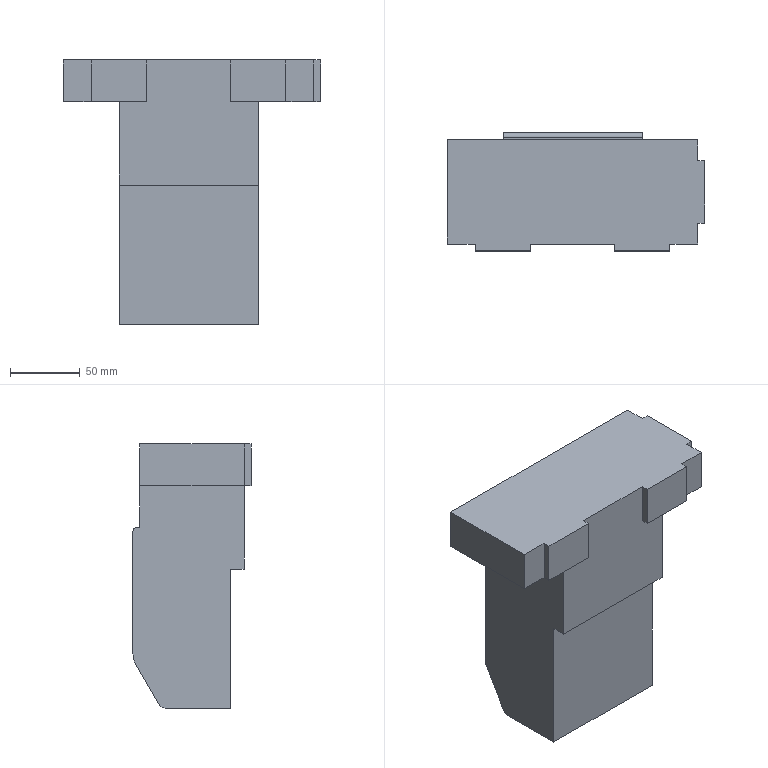Part | NX | features solid 2 | 1 solid | 30 faces | box 185 x 85 x 190 mm | volume 1552921 mm3 | plane 27 | cylinder 3 | commonest cylinder face diameters 6 x1 10 x1 30 x1
STEP:
#1=CARTESIAN_POINT('',(510.,415.,-90.));
#2=VERTEX_POINT('',#1);
#3=CARTESIAN_POINT('',(510.,415.,-120.));
#4=VERTEX_POINT('',#3);
#5=CARTESIAN_POINT('',(510.,415.,-90.));
#6=DIRECTION('',(0.,0.,-1.));
#7=VECTOR('',#6,1000.);
#8=LINE('',#5,#7);
#9=EDGE_CURVE('',#2,#4,#8,.T.);
#10=ORIENTED_EDGE('',*,*,#9,.F.);
#11=CARTESIAN_POINT('',(510.,400.,-90.));
#12=VERTEX_POINT('',#11);
#13=CARTESIAN_POINT('',(510.,475.,-90.));
#14=DIRECTION('',(0.,1.,0.));
#15=VECTOR('',#14,1000.);
#16=LINE('',#13,#15);
#17=EDGE_CURVE('',#2,#12,#16,.F.);
#18=ORIENTED_EDGE('',*,*,#17,.T.);
#19=CARTESIAN_POINT('',(510.,400.,-120.));
#20=VERTEX_POINT('',#19);
#21=CARTESIAN_POINT('',(510.,400.,-90.));
#22=DIRECTION('',(0.,0.,-1.));
#23=VECTOR('',#22,1000.);
#24=LINE('',#21,#23);
#25=EDGE_CURVE('',#12,#20,#24,.T.);
#26=ORIENTED_EDGE('',*,*,#25,.T.);
#27=CARTESIAN_POINT('',(510.,475.,-120.));
#28=DIRECTION('',(0.,1.,0.));
#29=VECTOR('',#28,1000.);
#30=LINE('',#27,#29);
#31=EDGE_CURVE('',#4,#20,#30,.F.);
#32=ORIENTED_EDGE('',*,*,#31,.F.);
#33=EDGE_LOOP('',(#10,#18,#26,#32));
#34=FACE_BOUND('',#33,.T.);
#35=CARTESIAN_POINT('',(510.,475.,-90.));
#36=DIRECTION('',(-1.,0.,0.));
#37=DIRECTION('',(0.,0.,-1.));
#38=AXIS2_PLACEMENT_3D('',#35,#36,#37);
#39=PLANE('',#38);
#40=ADVANCED_FACE('',(#34),#39,.F.);
#41=CARTESIAN_POINT('',(490.,400.,-120.));
#42=VERTEX_POINT('',#41);
#43=CARTESIAN_POINT('',(490.,400.,-90.));
#44=VERTEX_POINT('',#43);
#45=CARTESIAN_POINT('',(490.,400.,-180.));
#46=DIRECTION('',(0.,0.,1.));
#47=VECTOR('',#46,1000.);
#48=LINE('',#45,#47);
#49=EDGE_CURVE('',#42,#44,#48,.T.);
#50=ORIENTED_EDGE('',*,*,#49,.F.);
#51=CARTESIAN_POINT('',(470.,400.,-120.));
#52=DIRECTION('',(1.,0.,0.));
#53=VECTOR('',#52,1000.);
#54=LINE('',#51,#53);
#55=EDGE_CURVE('',#20,#42,#54,.F.);
#56=ORIENTED_EDGE('',*,*,#55,.F.);
#57=ORIENTED_EDGE('',*,*,#25,.F.);
#58=CARTESIAN_POINT('',(370.,400.,-90.));
#59=DIRECTION('',(1.,0.,0.));
#60=VECTOR('',#59,1000.);
#61=LINE('',#58,#60);
#62=EDGE_CURVE('',#44,#12,#61,.T.);
#63=ORIENTED_EDGE('',*,*,#62,.F.);
#64=EDGE_LOOP('',(#50,#56,#57,#63));
#65=FACE_BOUND('',#64,.T.);
#66=CARTESIAN_POINT('',(370.,400.,-180.));
#67=DIRECTION('',(0.,-1.,0.));
#68=DIRECTION('',(0.,0.,-1.));
#69=AXIS2_PLACEMENT_3D('',#66,#67,#68);
#70=PLANE('',#69);
#71=ADVANCED_FACE('',(#65),#70,.T.);
#72=CARTESIAN_POINT('',(330.,475.,-90.));
#73=VERTEX_POINT('',#72);
#74=CARTESIAN_POINT('',(510.,475.,-90.));
#75=VERTEX_POINT('',#74);
#76=CARTESIAN_POINT('',(370.,475.,-90.));
#77=DIRECTION('',(1.,0.,0.));
#78=VECTOR('',#77,1000.);
#79=LINE('',#76,#78);
#80=EDGE_CURVE('',#73,#75,#79,.T.);
#81=ORIENTED_EDGE('',*,*,#80,.T.);
#82=CARTESIAN_POINT('',(510.,475.,-120.));
#83=VERTEX_POINT('',#82);
#84=CARTESIAN_POINT('',(510.,475.,-90.));
#85=DIRECTION('',(0.,0.,-1.));
#86=VECTOR('',#85,1000.);
#87=LINE('',#84,#86);
#88=EDGE_CURVE('',#75,#83,#87,.T.);
#89=ORIENTED_EDGE('',*,*,#88,.T.);
#90=CARTESIAN_POINT('',(470.,475.,-120.));
#91=VERTEX_POINT('',#90);
#92=CARTESIAN_POINT('',(470.,475.,-120.));
#93=DIRECTION('',(1.,0.,0.));
#94=VECTOR('',#93,1000.);
#95=LINE('',#92,#94);
#96=EDGE_CURVE('',#83,#91,#95,.F.);
#97=ORIENTED_EDGE('',*,*,#96,.T.);
#98=CARTESIAN_POINT('',(470.,475.,-150.));
#99=VERTEX_POINT('',#98);
#100=CARTESIAN_POINT('',(470.,475.,-90.));
#101=DIRECTION('',(0.,0.,-1.));
#102=VECTOR('',#101,1000.);
#103=LINE('',#100,#102);
#104=EDGE_CURVE('',#91,#99,#103,.T.);
#105=ORIENTED_EDGE('',*,*,#104,.T.);
#106=CARTESIAN_POINT('',(370.,475.,-150.));
#107=VERTEX_POINT('',#106);
#108=CARTESIAN_POINT('',(370.,475.,-150.));
#109=DIRECTION('',(1.,0.,0.));
#110=VECTOR('',#109,1000.);
#111=LINE('',#108,#110);
#112=EDGE_CURVE('',#107,#99,#111,.T.);
#113=ORIENTED_EDGE('',*,*,#112,.F.);
#114=CARTESIAN_POINT('',(370.,475.,-120.));
#115=VERTEX_POINT('',#114);
#116=CARTESIAN_POINT('',(370.,475.,-90.));
#117=DIRECTION('',(0.,0.,-1.));
#118=VECTOR('',#117,1000.);
#119=LINE('',#116,#118);
#120=EDGE_CURVE('',#115,#107,#119,.T.);
#121=ORIENTED_EDGE('',*,*,#120,.F.);
#122=CARTESIAN_POINT('',(330.,475.,-120.));
#123=VERTEX_POINT('',#122);
#124=CARTESIAN_POINT('',(370.,475.,-120.));
#125=DIRECTION('',(1.,0.,0.));
#126=VECTOR('',#125,1000.);
#127=LINE('',#124,#126);
#128=EDGE_CURVE('',#123,#115,#127,.T.);
#129=ORIENTED_EDGE('',*,*,#128,.F.);
#130=CARTESIAN_POINT('',(330.,475.,-90.));
#131=DIRECTION('',(0.,0.,-1.));
#132=VECTOR('',#131,1000.);
#133=LINE('',#130,#132);
#134=EDGE_CURVE('',#73,#123,#133,.T.);
#135=ORIENTED_EDGE('',*,*,#134,.F.);
#136=EDGE_LOOP('',(#81,#89,#97,#105,#113,#121,#129,#135));
#137=FACE_BOUND('',#136,.T.);
#138=CARTESIAN_POINT('',(370.,475.,-90.));
#139=DIRECTION('',(0.,1.,0.));
#140=DIRECTION('',(0.,0.,1.));
#141=AXIS2_PLACEMENT_3D('',#138,#139,#140);
#142=PLANE('',#141);
#143=ADVANCED_FACE('',(#137),#142,.T.);
#144=ORIENTED_EDGE('',*,*,#80,.F.);
#145=CARTESIAN_POINT('',(330.,400.,-90.));
#146=VERTEX_POINT('',#145);
#147=CARTESIAN_POINT('',(330.,475.,-90.));
#148=DIRECTION('',(0.,1.,0.));
#149=VECTOR('',#148,1000.);
#150=LINE('',#147,#149);
#151=EDGE_CURVE('',#73,#146,#150,.F.);
#152=ORIENTED_EDGE('',*,*,#151,.T.);
#153=CARTESIAN_POINT('',(350.,400.,-90.));
#154=VERTEX_POINT('',#153);
#155=CARTESIAN_POINT('',(370.,400.,-90.));
#156=DIRECTION('',(1.,0.,0.));
#157=VECTOR('',#156,1000.);
#158=LINE('',#155,#157);
#159=EDGE_CURVE('',#146,#154,#158,.T.);
#160=ORIENTED_EDGE('',*,*,#159,.T.);
#161=CARTESIAN_POINT('',(350.,395.,-90.));
#162=VERTEX_POINT('',#161);
#163=CARTESIAN_POINT('',(350.,395.,-90.));
#164=DIRECTION('',(0.,1.,0.));
#165=VECTOR('',#164,1000.);
#166=LINE('',#163,#165);
#167=EDGE_CURVE('',#162,#154,#166,.T.);
#168=ORIENTED_EDGE('',*,*,#167,.F.);
#169=CARTESIAN_POINT('',(390.,395.,-90.));
#170=VERTEX_POINT('',#169);
#171=CARTESIAN_POINT('',(290.,395.,-90.));
#172=DIRECTION('',(1.,0.,0.));
#173=VECTOR('',#172,1000.);
#174=LINE('',#171,#173);
#175=EDGE_CURVE('',#162,#170,#174,.T.);
#176=ORIENTED_EDGE('',*,*,#175,.T.);
#177=CARTESIAN_POINT('',(390.,400.,-90.));
#178=VERTEX_POINT('',#177);
#179=CARTESIAN_POINT('',(390.,395.,-90.));
#180=DIRECTION('',(0.,1.,0.));
#181=VECTOR('',#180,1000.);
#182=LINE('',#179,#181);
#183=EDGE_CURVE('',#170,#178,#182,.T.);
#184=ORIENTED_EDGE('',*,*,#183,.T.);
#185=CARTESIAN_POINT('',(450.,400.,-90.));
#186=VERTEX_POINT('',#185);
#187=CARTESIAN_POINT('',(370.,400.,-90.));
#188=DIRECTION('',(1.,0.,0.));
#189=VECTOR('',#188,1000.);
#190=LINE('',#187,#189);
#191=EDGE_CURVE('',#178,#186,#190,.T.);
#192=ORIENTED_EDGE('',*,*,#191,.T.);
#193=CARTESIAN_POINT('',(450.,395.,-90.));
#194=VERTEX_POINT('',#193);
#195=CARTESIAN_POINT('',(450.,395.,-90.));
#196=DIRECTION('',(0.,1.,0.));
#197=VECTOR('',#196,1000.);
#198=LINE('',#195,#197);
#199=EDGE_CURVE('',#194,#186,#198,.T.);
#200=ORIENTED_EDGE('',*,*,#199,.F.);
#201=CARTESIAN_POINT('',(490.,395.,-90.));
#202=VERTEX_POINT('',#201);
#203=CARTESIAN_POINT('',(390.,395.,-90.));
#204=DIRECTION('',(1.,0.,0.));
#205=VECTOR('',#204,1000.);
#206=LINE('',#203,#205);
#207=EDGE_CURVE('',#194,#202,#206,.T.);
#208=ORIENTED_EDGE('',*,*,#207,.T.);
#209=CARTESIAN_POINT('',(490.,395.,-90.));
#210=DIRECTION('',(0.,1.,0.));
#211=VECTOR('',#210,1000.);
#212=LINE('',#209,#211);
#213=EDGE_CURVE('',#202,#44,#212,.T.);
#214=ORIENTED_EDGE('',*,*,#213,.T.);
#215=ORIENTED_EDGE('',*,*,#62,.T.);
#216=ORIENTED_EDGE('',*,*,#17,.F.);
#217=CARTESIAN_POINT('',(515.,415.,-90.));
#218=VERTEX_POINT('',#217);
#219=CARTESIAN_POINT('',(515.,415.,-90.));
#220=DIRECTION('',(-1.,0.,0.));
#221=VECTOR('',#220,1000.);
#222=LINE('',#219,#221);
#223=EDGE_CURVE('',#218,#2,#222,.T.);
#224=ORIENTED_EDGE('',*,*,#223,.F.);
#225=CARTESIAN_POINT('',(515.,460.,-90.));
#226=VERTEX_POINT('',#225);
#227=CARTESIAN_POINT('',(515.,475.,-90.));
#228=DIRECTION('',(0.,1.,0.));
#229=VECTOR('',#228,1000.);
#230=LINE('',#227,#229);
#231=EDGE_CURVE('',#226,#218,#230,.F.);
#232=ORIENTED_EDGE('',*,*,#231,.F.);
#233=CARTESIAN_POINT('',(510.,460.,-90.));
#234=VERTEX_POINT('',#233);
#235=CARTESIAN_POINT('',(515.,460.,-90.));
#236=DIRECTION('',(-1.,0.,0.));
#237=VECTOR('',#236,1000.);
#238=LINE('',#235,#237);
#239=EDGE_CURVE('',#226,#234,#238,.T.);
#240=ORIENTED_EDGE('',*,*,#239,.T.);
#241=CARTESIAN_POINT('',(510.,475.,-90.));
#242=DIRECTION('',(0.,1.,0.));
#243=VECTOR('',#242,1000.);
#244=LINE('',#241,#243);
#245=EDGE_CURVE('',#75,#234,#244,.F.);
#246=ORIENTED_EDGE('',*,*,#245,.F.);
#247=EDGE_LOOP('',(#144,#152,#160,#168,#176,#184,#192,#200,#208,#214,#215,#216,#224,#232,#240,#246));
#248=FACE_BOUND('',#247,.T.);
#249=CARTESIAN_POINT('',(370.,475.,-90.));
#250=DIRECTION('',(0.,0.,-1.));
#251=DIRECTION('',(1.,0.,0.));
#252=AXIS2_PLACEMENT_3D('',#249,#250,#251);
#253=PLANE('',#252);
#254=ADVANCED_FACE('',(#248),#253,.F.);
#255=CARTESIAN_POINT('',(390.,400.,-120.));
#256=VERTEX_POINT('',#255);
#257=CARTESIAN_POINT('',(390.,400.,-180.));
#258=DIRECTION('',(0.,0.,1.));
#259=VECTOR('',#258,1000.);
#260=LINE('',#257,#259);
#261=EDGE_CURVE('',#256,#178,#260,.T.);
#262=ORIENTED_EDGE('',*,*,#261,.F.);
#263=CARTESIAN_POINT('',(370.,400.,-120.));
#264=VERTEX_POINT('',#263);
#265=CARTESIAN_POINT('',(290.,400.,-120.));
#266=DIRECTION('',(1.,0.,0.));
#267=VECTOR('',#266,1000.);
#268=LINE('',#265,#267);
#269=EDGE_CURVE('',#264,#256,#268,.T.);
#270=ORIENTED_EDGE('',*,*,#269,.F.);
#271=CARTESIAN_POINT('',(370.,400.,-180.));
#272=VERTEX_POINT('',#271);
#273=CARTESIAN_POINT('',(370.,400.,-180.));
#274=DIRECTION('',(0.,0.,1.));
#275=VECTOR('',#274,1000.);
#276=LINE('',#273,#275);
#277=EDGE_CURVE('',#272,#264,#276,.T.);
#278=ORIENTED_EDGE('',*,*,#277,.F.);
#279=CARTESIAN_POINT('',(470.,400.,-180.));
#280=VERTEX_POINT('',#279);
#281=CARTESIAN_POINT('',(370.,400.,-180.));
#282=DIRECTION('',(1.,0.,0.));
#283=VECTOR('',#282,1000.);
#284=LINE('',#281,#283);
#285=EDGE_CURVE('',#272,#280,#284,.T.);
#286=ORIENTED_EDGE('',*,*,#285,.T.);
#287=CARTESIAN_POINT('',(470.,400.,-120.));
#288=VERTEX_POINT('',#287);
#289=CARTESIAN_POINT('',(470.,400.,-180.));
#290=DIRECTION('',(0.,0.,1.));
#291=VECTOR('',#290,1000.);
#292=LINE('',#289,#291);
#293=EDGE_CURVE('',#280,#288,#292,.T.);
#294=ORIENTED_EDGE('',*,*,#293,.T.);
#295=CARTESIAN_POINT('',(450.,400.,-120.));
#296=VERTEX_POINT('',#295);
#297=CARTESIAN_POINT('',(390.,400.,-120.));
#298=DIRECTION('',(1.,0.,0.));
#299=VECTOR('',#298,1000.);
#300=LINE('',#297,#299);
#301=EDGE_CURVE('',#296,#288,#300,.T.);
#302=ORIENTED_EDGE('',*,*,#301,.F.);
#303=CARTESIAN_POINT('',(450.,400.,-180.));
#304=DIRECTION('',(0.,0.,1.));
#305=VECTOR('',#304,1000.);
#306=LINE('',#303,#305);
#307=EDGE_CURVE('',#296,#186,#306,.T.);
#308=ORIENTED_EDGE('',*,*,#307,.T.);
#309=ORIENTED_EDGE('',*,*,#191,.F.);
#310=EDGE_LOOP('',(#262,#270,#278,#286,#294,#302,#308,#309));
#311=FACE_BOUND('',#310,.T.);
#312=CARTESIAN_POINT('',(370.,400.,-180.));
#313=DIRECTION('',(0.,-1.,0.));
#314=DIRECTION('',(0.,0.,-1.));
#315=AXIS2_PLACEMENT_3D('',#312,#313,#314);
#316=PLANE('',#315);
#317=ADVANCED_FACE('',(#311),#316,.T.);
#318=CARTESIAN_POINT('',(470.,410.,-180.));
#319=VERTEX_POINT('',#318);
#320=CARTESIAN_POINT('',(470.,410.,-180.));
#321=DIRECTION('',(0.,-1.,0.));
#322=VECTOR('',#321,1000.);
#323=LINE('',#320,#322);
#324=EDGE_CURVE('',#319,#280,#323,.T.);
#325=ORIENTED_EDGE('',*,*,#324,.T.);
#326=ORIENTED_EDGE('',*,*,#285,.F.);
#327=CARTESIAN_POINT('',(370.,410.,-180.));
#328=VERTEX_POINT('',#327);
#329=CARTESIAN_POINT('',(370.,410.,-180.));
#330=DIRECTION('',(0.,-1.,0.));
#331=VECTOR('',#330,1000.);
#332=LINE('',#329,#331);
#333=EDGE_CURVE('',#328,#272,#332,.T.);
#334=ORIENTED_EDGE('',*,*,#333,.F.);
#335=CARTESIAN_POINT('',(370.,410.,-180.));
#336=DIRECTION('',(1.,0.,0.));
#337=VECTOR('',#336,1000.);
#338=LINE('',#335,#337);
#339=EDGE_CURVE('',#328,#319,#338,.T.);
#340=ORIENTED_EDGE('',*,*,#339,.T.);
#341=EDGE_LOOP('',(#325,#326,#334,#340));
#342=FACE_BOUND('',#341,.T.);
#343=CARTESIAN_POINT('',(370.,410.,-180.));
#344=DIRECTION('',(0.,0.,-1.));
#345=DIRECTION('',(0.,1.,0.));
#346=AXIS2_PLACEMENT_3D('',#343,#344,#345);
#347=PLANE('',#346);
#348=ADVANCED_FACE('',(#342),#347,.T.);
#349=CARTESIAN_POINT('',(470.,410.,-280.));
#350=VERTEX_POINT('',#349);
#351=CARTESIAN_POINT('',(470.,410.,-180.));
#352=DIRECTION('',(0.,0.,-1.));
#353=VECTOR('',#352,1000.);
#354=LINE('',#351,#353);
#355=EDGE_CURVE('',#319,#350,#354,.T.);
#356=ORIENTED_EDGE('',*,*,#355,.F.);
#357=ORIENTED_EDGE('',*,*,#339,.F.);
#358=CARTESIAN_POINT('',(370.,410.,-280.));
#359=VERTEX_POINT('',#358);
#360=CARTESIAN_POINT('',(370.,410.,-180.));
#361=DIRECTION('',(0.,0.,-1.));
#362=VECTOR('',#361,1000.);
#363=LINE('',#360,#362);
#364=EDGE_CURVE('',#328,#359,#363,.T.);
#365=ORIENTED_EDGE('',*,*,#364,.T.);
#366=CARTESIAN_POINT('',(370.,410.,-280.));
#367=DIRECTION('',(1.,0.,0.));
#368=VECTOR('',#367,1000.);
#369=LINE('',#366,#368);
#370=EDGE_CURVE('',#359,#350,#369,.T.);
#371=ORIENTED_EDGE('',*,*,#370,.T.);
#372=EDGE_LOOP('',(#356,#357,#365,#371));
#373=FACE_BOUND('',#372,.T.);
#374=CARTESIAN_POINT('',(370.,410.,-180.));
#375=DIRECTION('',(0.,1.,0.));
#376=DIRECTION('',(0.,0.,1.));
#377=AXIS2_PLACEMENT_3D('',#374,#375,#376);
#378=PLANE('',#377);
#379=ADVANCED_FACE('',(#373),#378,.F.);
#380=CARTESIAN_POINT('',(470.,456.906,-280.));
#381=VERTEX_POINT('',#380);
#382=CARTESIAN_POINT('',(470.,450.,-280.));
#383=DIRECTION('',(0.,-1.,0.));
#384=VECTOR('',#383,1000.);
#385=LINE('',#382,#384);
#386=EDGE_CURVE('',#381,#350,#385,.T.);
#387=ORIENTED_EDGE('',*,*,#386,.T.);
#388=ORIENTED_EDGE('',*,*,#370,.F.);
#389=CARTESIAN_POINT('',(370.,456.906,-280.));
#390=VERTEX_POINT('',#389);
#391=CARTESIAN_POINT('',(370.,450.,-280.));
#392=DIRECTION('',(0.,-1.,0.));
#393=VECTOR('',#392,1000.);
#394=LINE('',#391,#393);
#395=EDGE_CURVE('',#390,#359,#394,.T.);
#396=ORIENTED_EDGE('',*,*,#395,.F.);
#397=CARTESIAN_POINT('',(370.,456.906,-280.));
#398=DIRECTION('',(1.,0.,0.));
#399=VECTOR('',#398,1000.);
#400=LINE('',#397,#399);
#401=EDGE_CURVE('',#390,#381,#400,.T.);
#402=ORIENTED_EDGE('',*,*,#401,.T.);
#403=EDGE_LOOP('',(#387,#388,#396,#402));
#404=FACE_BOUND('',#403,.T.);
#405=CARTESIAN_POINT('',(370.,450.,-280.));
#406=DIRECTION('',(0.,0.,-1.));
#407=DIRECTION('',(0.,1.,0.));
#408=AXIS2_PLACEMENT_3D('',#405,#406,#407);
#409=PLANE('',#408);
#410=ADVANCED_FACE('',(#404),#409,.T.);
#411=CARTESIAN_POINT('',(370.,475.,-120.));
#412=DIRECTION('',(0.,-1.,0.));
#413=VECTOR('',#412,1000.);
#414=LINE('',#411,#413);
#415=EDGE_CURVE('',#115,#264,#414,.T.);
#416=ORIENTED_EDGE('',*,*,#415,.F.);
#417=ORIENTED_EDGE('',*,*,#120,.T.);
#418=CARTESIAN_POINT('',(370.,477.,-150.));
#419=VERTEX_POINT('',#418);
#420=CARTESIAN_POINT('',(370.,450.,-150.));
#421=DIRECTION('',(0.,1.,0.));
#422=VECTOR('',#421,1000.);
#423=LINE('',#420,#422);
#424=EDGE_CURVE('',#107,#419,#423,.T.);
#425=ORIENTED_EDGE('',*,*,#424,.T.);
#426=CARTESIAN_POINT('',(370.,480.,-153.));
#427=VERTEX_POINT('',#426);
#428=CARTESIAN_POINT('',(370.,477.,-153.));
#429=DIRECTION('',(1.,0.,0.));
#430=DIRECTION('',(0.,-1.,0.));
#431=AXIS2_PLACEMENT_3D('',#428,#429,#430);
#432=CIRCLE('',#431,3.);
#433=EDGE_CURVE('',#427,#419,#432,.T.);
#434=ORIENTED_EDGE('',*,*,#433,.F.);
#435=CARTESIAN_POINT('',(370.,480.,-240.981));
#436=VERTEX_POINT('',#435);
#437=CARTESIAN_POINT('',(370.,480.,-153.));
#438=DIRECTION('',(0.,0.,-1.));
#439=VECTOR('',#438,1000.);
#440=LINE('',#437,#439);
#441=EDGE_CURVE('',#427,#436,#440,.T.);
#442=ORIENTED_EDGE('',*,*,#441,.T.);
#443=CARTESIAN_POINT('',(370.,477.99,-248.481));
#444=VERTEX_POINT('',#443);
#445=CARTESIAN_POINT('',(370.,465.,-240.981));
#446=DIRECTION('',(1.,0.,0.));
#447=DIRECTION('',(0.,-1.,0.));
#448=AXIS2_PLACEMENT_3D('',#445,#446,#447);
#449=CIRCLE('',#448,15.);
#450=EDGE_CURVE('',#444,#436,#449,.T.);
#451=ORIENTED_EDGE('',*,*,#450,.F.);
#452=CARTESIAN_POINT('',(370.,461.236,-277.5));
#453=VERTEX_POINT('',#452);
#454=CARTESIAN_POINT('',(370.,480.,-245.));
#455=DIRECTION('',(0.,-0.5,-0.866));
#456=VECTOR('',#455,1000.);
#457=LINE('',#454,#456);
#458=EDGE_CURVE('',#444,#453,#457,.T.);
#459=ORIENTED_EDGE('',*,*,#458,.T.);
#460=CARTESIAN_POINT('',(370.,456.906,-275.));
#461=DIRECTION('',(1.,0.,0.));
#462=DIRECTION('',(0.,-1.,0.));
#463=AXIS2_PLACEMENT_3D('',#460,#461,#462);
#464=CIRCLE('',#463,5.);
#465=EDGE_CURVE('',#390,#453,#464,.T.);
#466=ORIENTED_EDGE('',*,*,#465,.F.);
#467=ORIENTED_EDGE('',*,*,#395,.T.);
#468=ORIENTED_EDGE('',*,*,#364,.F.);
#469=ORIENTED_EDGE('',*,*,#333,.T.);
#470=ORIENTED_EDGE('',*,*,#277,.T.);
#471=EDGE_LOOP('',(#416,#417,#425,#434,#442,#451,#459,#466,#467,#468,#469,#470));
#472=FACE_BOUND('',#471,.T.);
#473=CARTESIAN_POINT('',(370.,443.375,-175.));
#474=DIRECTION('',(-1.,0.,0.));
#475=DIRECTION('',(0.,0.,-1.));
#476=AXIS2_PLACEMENT_3D('',#473,#474,#475);
#477=PLANE('',#476);
#478=ADVANCED_FACE('',(#472),#477,.T.);
#479=ORIENTED_EDGE('',*,*,#104,.F.);
#480=CARTESIAN_POINT('',(470.,475.,-120.));
#481=DIRECTION('',(0.,-1.,0.));
#482=VECTOR('',#481,1000.);
#483=LINE('',#480,#482);
#484=EDGE_CURVE('',#91,#288,#483,.T.);
#485=ORIENTED_EDGE('',*,*,#484,.T.);
#486=ORIENTED_EDGE('',*,*,#293,.F.);
#487=ORIENTED_EDGE('',*,*,#324,.F.);
#488=ORIENTED_EDGE('',*,*,#355,.T.);
#489=ORIENTED_EDGE('',*,*,#386,.F.);
#490=CARTESIAN_POINT('',(470.,461.236,-277.5));
#491=VERTEX_POINT('',#490);
#492=CARTESIAN_POINT('',(470.,456.906,-275.));
#493=DIRECTION('',(1.,0.,0.));
#494=DIRECTION('',(0.,-1.,0.));
#495=AXIS2_PLACEMENT_3D('',#492,#493,#494);
#496=CIRCLE('',#495,5.);
#497=EDGE_CURVE('',#381,#491,#496,.T.);
#498=ORIENTED_EDGE('',*,*,#497,.T.);
#499=CARTESIAN_POINT('',(470.,477.99,-248.481));
#500=VERTEX_POINT('',#499);
#501=CARTESIAN_POINT('',(470.,480.,-245.));
#502=DIRECTION('',(0.,-0.5,-0.866));
#503=VECTOR('',#502,1000.);
#504=LINE('',#501,#503);
#505=EDGE_CURVE('',#500,#491,#504,.T.);
#506=ORIENTED_EDGE('',*,*,#505,.F.);
#507=CARTESIAN_POINT('',(470.,480.,-240.981));
#508=VERTEX_POINT('',#507);
#509=CARTESIAN_POINT('',(470.,465.,-240.981));
#510=DIRECTION('',(1.,0.,0.));
#511=DIRECTION('',(0.,-1.,0.));
#512=AXIS2_PLACEMENT_3D('',#509,#510,#511);
#513=CIRCLE('',#512,15.);
#514=EDGE_CURVE('',#500,#508,#513,.T.);
#515=ORIENTED_EDGE('',*,*,#514,.T.);
#516=CARTESIAN_POINT('',(470.,480.,-153.));
#517=VERTEX_POINT('',#516);
#518=CARTESIAN_POINT('',(470.,480.,-153.));
#519=DIRECTION('',(0.,0.,-1.));
#520=VECTOR('',#519,1000.);
#521=LINE('',#518,#520);
#522=EDGE_CURVE('',#517,#508,#521,.T.);
#523=ORIENTED_EDGE('',*,*,#522,.F.);
#524=CARTESIAN_POINT('',(470.,477.,-150.));
#525=VERTEX_POINT('',#524);
#526=CARTESIAN_POINT('',(470.,477.,-153.));
#527=DIRECTION('',(1.,0.,0.));
#528=DIRECTION('',(0.,-1.,0.));
#529=AXIS2_PLACEMENT_3D('',#526,#527,#528);
#530=CIRCLE('',#529,3.);
#531=EDGE_CURVE('',#517,#525,#530,.T.);
#532=ORIENTED_EDGE('',*,*,#531,.T.);
#533=CARTESIAN_POINT('',(470.,450.,-150.));
#534=DIRECTION('',(0.,1.,0.));
#535=VECTOR('',#534,1000.);
#536=LINE('',#533,#535);
#537=EDGE_CURVE('',#99,#525,#536,.T.);
#538=ORIENTED_EDGE('',*,*,#537,.F.);
#539=EDGE_LOOP('',(#479,#485,#486,#487,#488,#489,#498,#506,#515,#523,#532,#538));
#540=FACE_BOUND('',#539,.T.);
#541=CARTESIAN_POINT('',(470.,443.375,-175.));
#542=DIRECTION('',(-1.,0.,0.));
#543=DIRECTION('',(0.,0.,-1.));
#544=AXIS2_PLACEMENT_3D('',#541,#542,#543);
#545=PLANE('',#544);
#546=ADVANCED_FACE('',(#540),#545,.F.);
#547=ORIENTED_EDGE('',*,*,#497,.F.);
#548=ORIENTED_EDGE('',*,*,#401,.F.);
#549=ORIENTED_EDGE('',*,*,#465,.T.);
#550=CARTESIAN_POINT('',(370.,461.236,-277.5));
#551=DIRECTION('',(1.,0.,0.));
#552=VECTOR('',#551,1000.);
#553=LINE('',#550,#552);
#554=EDGE_CURVE('',#453,#491,#553,.T.);
#555=ORIENTED_EDGE('',*,*,#554,.T.);
#556=EDGE_LOOP('',(#547,#548,#549,#555));
#557=FACE_BOUND('',#556,.T.);
#558=CARTESIAN_POINT('',(370.,456.906,-275.));
#559=DIRECTION('',(1.,0.,0.));
#560=DIRECTION('',(0.,0.,1.));
#561=AXIS2_PLACEMENT_3D('',#558,#559,#560);
#562=CYLINDRICAL_SURFACE('',#561,5.);
#563=ADVANCED_FACE('',(#557),#562,.T.);
#564=ORIENTED_EDGE('',*,*,#505,.T.);
#565=ORIENTED_EDGE('',*,*,#554,.F.);
#566=ORIENTED_EDGE('',*,*,#458,.F.);
#567=CARTESIAN_POINT('',(370.,477.99,-248.481));
#568=DIRECTION('',(1.,0.,0.));
#569=VECTOR('',#568,1000.);
#570=LINE('',#567,#569);
#571=EDGE_CURVE('',#444,#500,#570,.T.);
#572=ORIENTED_EDGE('',*,*,#571,.T.);
#573=EDGE_LOOP('',(#564,#565,#566,#572));
#574=FACE_BOUND('',#573,.T.);
#575=CARTESIAN_POINT('',(370.,480.,-245.));
#576=DIRECTION('',(0.,0.866,-0.5));
#577=DIRECTION('',(0.,0.5,0.866));
#578=AXIS2_PLACEMENT_3D('',#575,#576,#577);
#579=PLANE('',#578);
#580=ADVANCED_FACE('',(#574),#579,.T.);
#581=ORIENTED_EDGE('',*,*,#514,.F.);
#582=ORIENTED_EDGE('',*,*,#571,.F.);
#583=ORIENTED_EDGE('',*,*,#450,.T.);
#584=CARTESIAN_POINT('',(370.,480.,-240.981));
#585=DIRECTION('',(1.,0.,0.));
#586=VECTOR('',#585,1000.);
#587=LINE('',#584,#586);
#588=EDGE_CURVE('',#436,#508,#587,.T.);
#589=ORIENTED_EDGE('',*,*,#588,.T.);
#590=EDGE_LOOP('',(#581,#582,#583,#589));
#591=FACE_BOUND('',#590,.T.);
#592=CARTESIAN_POINT('',(370.,465.,-240.981));
#593=DIRECTION('',(1.,0.,0.));
#594=DIRECTION('',(0.,0.,1.));
#595=AXIS2_PLACEMENT_3D('',#592,#593,#594);
#596=CYLINDRICAL_SURFACE('',#595,15.);
#597=ADVANCED_FACE('',(#591),#596,.T.);
#598=ORIENTED_EDGE('',*,*,#522,.T.);
#599=ORIENTED_EDGE('',*,*,#588,.F.);
#600=ORIENTED_EDGE('',*,*,#441,.F.);
#601=CARTESIAN_POINT('',(370.,480.,-153.));
#602=DIRECTION('',(1.,0.,0.));
#603=VECTOR('',#602,1000.);
#604=LINE('',#601,#603);
#605=EDGE_CURVE('',#427,#517,#604,.T.);
#606=ORIENTED_EDGE('',*,*,#605,.T.);
#607=EDGE_LOOP('',(#598,#599,#600,#606));
#608=FACE_BOUND('',#607,.T.);
#609=CARTESIAN_POINT('',(370.,480.,-153.));
#610=DIRECTION('',(0.,1.,0.));
#611=DIRECTION('',(0.,0.,1.));
#612=AXIS2_PLACEMENT_3D('',#609,#610,#611);
#613=PLANE('',#612);
#614=ADVANCED_FACE('',(#608),#613,.T.);
#615=ORIENTED_EDGE('',*,*,#531,.F.);
#616=ORIENTED_EDGE('',*,*,#605,.F.);
#617=ORIENTED_EDGE('',*,*,#433,.T.);
#618=CARTESIAN_POINT('',(370.,477.,-150.));
#619=DIRECTION('',(1.,0.,0.));
#620=VECTOR('',#619,1000.);
#621=LINE('',#618,#620);
#622=EDGE_CURVE('',#419,#525,#621,.T.);
#623=ORIENTED_EDGE('',*,*,#622,.T.);
#624=EDGE_LOOP('',(#615,#616,#617,#623));
#625=FACE_BOUND('',#624,.T.);
#626=CARTESIAN_POINT('',(370.,477.,-153.));
#627=DIRECTION('',(1.,0.,0.));
#628=DIRECTION('',(0.,0.,1.));
#629=AXIS2_PLACEMENT_3D('',#626,#627,#628);
#630=CYLINDRICAL_SURFACE('',#629,3.);
#631=ADVANCED_FACE('',(#625),#630,.T.);
#632=ORIENTED_EDGE('',*,*,#537,.T.);
#633=ORIENTED_EDGE('',*,*,#622,.F.);
#634=ORIENTED_EDGE('',*,*,#424,.F.);
#635=ORIENTED_EDGE('',*,*,#112,.T.);
#636=EDGE_LOOP('',(#632,#633,#634,#635));
#637=FACE_BOUND('',#636,.T.);
#638=CARTESIAN_POINT('',(370.,450.,-150.));
#639=DIRECTION('',(0.,0.,1.));
#640=DIRECTION('',(0.,-1.,0.));
#641=AXIS2_PLACEMENT_3D('',#638,#639,#640);
#642=PLANE('',#641);
#643=ADVANCED_FACE('',(#637),#642,.T.);
#644=ORIENTED_EDGE('',*,*,#96,.F.);
#645=CARTESIAN_POINT('',(510.,460.,-120.));
#646=VERTEX_POINT('',#645);
#647=CARTESIAN_POINT('',(510.,475.,-120.));
#648=DIRECTION('',(0.,1.,0.));
#649=VECTOR('',#648,1000.);
#650=LINE('',#647,#649);
#651=EDGE_CURVE('',#83,#646,#650,.F.);
#652=ORIENTED_EDGE('',*,*,#651,.T.);
#653=CARTESIAN_POINT('',(515.,460.,-120.));
#654=VERTEX_POINT('',#653);
#655=CARTESIAN_POINT('',(515.,460.,-120.));
#656=DIRECTION('',(-1.,0.,0.));
#657=VECTOR('',#656,1000.);
#658=LINE('',#655,#657);
#659=EDGE_CURVE('',#654,#646,#658,.T.);
#660=ORIENTED_EDGE('',*,*,#659,.F.);
#661=CARTESIAN_POINT('',(515.,415.,-120.));
#662=VERTEX_POINT('',#661);
#663=CARTESIAN_POINT('',(515.,475.,-120.));
#664=DIRECTION('',(0.,1.,0.));
#665=VECTOR('',#664,1000.);
#666=LINE('',#663,#665);
#667=EDGE_CURVE('',#654,#662,#666,.F.);
#668=ORIENTED_EDGE('',*,*,#667,.T.);
#669=CARTESIAN_POINT('',(515.,415.,-120.));
#670=DIRECTION('',(-1.,0.,0.));
#671=VECTOR('',#670,1000.);
#672=LINE('',#669,#671);
#673=EDGE_CURVE('',#662,#4,#672,.T.);
#674=ORIENTED_EDGE('',*,*,#673,.T.);
#675=ORIENTED_EDGE('',*,*,#31,.T.);
#676=ORIENTED_EDGE('',*,*,#55,.T.);
#677=CARTESIAN_POINT('',(490.,395.,-120.));
#678=VERTEX_POINT('',#677);
#679=CARTESIAN_POINT('',(490.,395.,-120.));
#680=DIRECTION('',(0.,1.,0.));
#681=VECTOR('',#680,1000.);
#682=LINE('',#679,#681);
#683=EDGE_CURVE('',#678,#42,#682,.T.);
#684=ORIENTED_EDGE('',*,*,#683,.F.);
#685=CARTESIAN_POINT('',(450.,395.,-120.));
#686=VERTEX_POINT('',#685);
#687=CARTESIAN_POINT('',(390.,395.,-120.));
#688=DIRECTION('',(1.,0.,0.));
#689=VECTOR('',#688,1000.);
#690=LINE('',#687,#689);
#691=EDGE_CURVE('',#686,#678,#690,.T.);
#692=ORIENTED_EDGE('',*,*,#691,.F.);
#693=CARTESIAN_POINT('',(450.,395.,-120.));
#694=DIRECTION('',(0.,1.,0.));
#695=VECTOR('',#694,1000.);
#696=LINE('',#693,#695);
#697=EDGE_CURVE('',#686,#296,#696,.T.);
#698=ORIENTED_EDGE('',*,*,#697,.T.);
#699=ORIENTED_EDGE('',*,*,#301,.T.);
#700=ORIENTED_EDGE('',*,*,#484,.F.);
#701=EDGE_LOOP('',(#644,#652,#660,#668,#674,#675,#676,#684,#692,#698,#699,#700));
#702=FACE_BOUND('',#701,.T.);
#703=CARTESIAN_POINT('',(470.,475.,-120.));
#704=DIRECTION('',(0.,0.,1.));
#705=DIRECTION('',(0.,-1.,0.));
#706=AXIS2_PLACEMENT_3D('',#703,#704,#705);
#707=PLANE('',#706);
#708=ADVANCED_FACE('',(#702),#707,.F.);
#709=ORIENTED_EDGE('',*,*,#245,.T.);
#710=CARTESIAN_POINT('',(510.,460.,-90.));
#711=DIRECTION('',(0.,0.,-1.));
#712=VECTOR('',#711,1000.);
#713=LINE('',#710,#712);
#714=EDGE_CURVE('',#234,#646,#713,.T.);
#715=ORIENTED_EDGE('',*,*,#714,.T.);
#716=ORIENTED_EDGE('',*,*,#651,.F.);
#717=ORIENTED_EDGE('',*,*,#88,.F.);
#718=EDGE_LOOP('',(#709,#715,#716,#717));
#719=FACE_BOUND('',#718,.T.);
#720=CARTESIAN_POINT('',(510.,475.,-90.));
#721=DIRECTION('',(-1.,0.,0.));
#722=DIRECTION('',(0.,0.,-1.));
#723=AXIS2_PLACEMENT_3D('',#720,#721,#722);
#724=PLANE('',#723);
#725=ADVANCED_FACE('',(#719),#724,.F.);
#726=ORIENTED_EDGE('',*,*,#49,.T.);
#727=ORIENTED_EDGE('',*,*,#213,.F.);
#728=CARTESIAN_POINT('',(490.,395.,-180.));
#729=DIRECTION('',(0.,0.,1.));
#730=VECTOR('',#729,1000.);
#731=LINE('',#728,#730);
#732=EDGE_CURVE('',#678,#202,#731,.T.);
#733=ORIENTED_EDGE('',*,*,#732,.F.);
#734=ORIENTED_EDGE('',*,*,#683,.T.);
#735=EDGE_LOOP('',(#726,#727,#733,#734));
#736=FACE_BOUND('',#735,.T.);
#737=CARTESIAN_POINT('',(490.,395.,-180.));
#738=DIRECTION('',(1.,0.,0.));
#739=DIRECTION('',(0.,0.,1.));
#740=AXIS2_PLACEMENT_3D('',#737,#738,#739);
#741=PLANE('',#740);
#742=ADVANCED_FACE('',(#736),#741,.T.);
#743=ORIENTED_EDGE('',*,*,#307,.F.);
#744=ORIENTED_EDGE('',*,*,#697,.F.);
#745=CARTESIAN_POINT('',(450.,395.,-180.));
#746=DIRECTION('',(0.,0.,1.));
#747=VECTOR('',#746,1000.);
#748=LINE('',#745,#747);
#749=EDGE_CURVE('',#686,#194,#748,.T.);
#750=ORIENTED_EDGE('',*,*,#749,.T.);
#751=ORIENTED_EDGE('',*,*,#199,.T.);
#752=EDGE_LOOP('',(#743,#744,#750,#751));
#753=FACE_BOUND('',#752,.T.);
#754=CARTESIAN_POINT('',(450.,395.,-180.));
#755=DIRECTION('',(1.,0.,0.));
#756=DIRECTION('',(0.,0.,1.));
#757=AXIS2_PLACEMENT_3D('',#754,#755,#756);
#758=PLANE('',#757);
#759=ADVANCED_FACE('',(#753),#758,.F.);
#760=ORIENTED_EDGE('',*,*,#732,.T.);
#761=ORIENTED_EDGE('',*,*,#207,.F.);
#762=ORIENTED_EDGE('',*,*,#749,.F.);
#763=ORIENTED_EDGE('',*,*,#691,.T.);
#764=EDGE_LOOP('',(#760,#761,#762,#763));
#765=FACE_BOUND('',#764,.T.);
#766=CARTESIAN_POINT('',(390.,395.,-180.));
#767=DIRECTION('',(0.,-1.,0.));
#768=DIRECTION('',(0.,0.,-1.));
#769=AXIS2_PLACEMENT_3D('',#766,#767,#768);
#770=PLANE('',#769);
#771=ADVANCED_FACE('',(#765),#770,.T.);
#772=ORIENTED_EDGE('',*,*,#261,.T.);
#773=ORIENTED_EDGE('',*,*,#183,.F.);
#774=CARTESIAN_POINT('',(390.,395.,-120.));
#775=VERTEX_POINT('',#774);
#776=CARTESIAN_POINT('',(390.,395.,-180.));
#777=DIRECTION('',(0.,0.,1.));
#778=VECTOR('',#777,1000.);
#779=LINE('',#776,#778);
#780=EDGE_CURVE('',#775,#170,#779,.T.);
#781=ORIENTED_EDGE('',*,*,#780,.F.);
#782=CARTESIAN_POINT('',(390.,395.,-120.));
#783=DIRECTION('',(0.,1.,0.));
#784=VECTOR('',#783,1000.);
#785=LINE('',#782,#784);
#786=EDGE_CURVE('',#775,#256,#785,.T.);
#787=ORIENTED_EDGE('',*,*,#786,.T.);
#788=EDGE_LOOP('',(#772,#773,#781,#787));
#789=FACE_BOUND('',#788,.T.);
#790=CARTESIAN_POINT('',(390.,395.,-180.));
#791=DIRECTION('',(1.,0.,0.));
#792=DIRECTION('',(0.,0.,1.));
#793=AXIS2_PLACEMENT_3D('',#790,#791,#792);
#794=PLANE('',#793);
#795=ADVANCED_FACE('',(#789),#794,.T.);
#796=CARTESIAN_POINT('',(350.,395.,-120.));
#797=VERTEX_POINT('',#796);
#798=CARTESIAN_POINT('',(350.,400.,-120.));
#799=VERTEX_POINT('',#798);
#800=CARTESIAN_POINT('',(350.,395.,-120.));
#801=DIRECTION('',(0.,1.,0.));
#802=VECTOR('',#801,1000.);
#803=LINE('',#800,#802);
#804=EDGE_CURVE('',#797,#799,#803,.T.);
#805=ORIENTED_EDGE('',*,*,#804,.T.);
#806=CARTESIAN_POINT('',(330.,400.,-120.));
#807=VERTEX_POINT('',#806);
#808=CARTESIAN_POINT('',(370.,400.,-120.));
#809=DIRECTION('',(1.,0.,0.));
#810=VECTOR('',#809,1000.);
#811=LINE('',#808,#810);
#812=EDGE_CURVE('',#807,#799,#811,.T.);
#813=ORIENTED_EDGE('',*,*,#812,.F.);
#814=CARTESIAN_POINT('',(330.,475.,-120.));
#815=DIRECTION('',(0.,1.,0.));
#816=VECTOR('',#815,1000.);
#817=LINE('',#814,#816);
#818=EDGE_CURVE('',#123,#807,#817,.F.);
#819=ORIENTED_EDGE('',*,*,#818,.F.);
#820=ORIENTED_EDGE('',*,*,#128,.T.);
#821=ORIENTED_EDGE('',*,*,#415,.T.);
#822=ORIENTED_EDGE('',*,*,#269,.T.);
#823=ORIENTED_EDGE('',*,*,#786,.F.);
#824=CARTESIAN_POINT('',(290.,395.,-120.));
#825=DIRECTION('',(1.,0.,0.));
#826=VECTOR('',#825,1000.);
#827=LINE('',#824,#826);
#828=EDGE_CURVE('',#797,#775,#827,.T.);
#829=ORIENTED_EDGE('',*,*,#828,.F.);
#830=EDGE_LOOP('',(#805,#813,#819,#820,#821,#822,#823,#829));
#831=FACE_BOUND('',#830,.T.);
#832=CARTESIAN_POINT('',(290.,395.,-120.));
#833=DIRECTION('',(0.,0.,-1.));
#834=DIRECTION('',(1.,0.,0.));
#835=AXIS2_PLACEMENT_3D('',#832,#833,#834);
#836=PLANE('',#835);
#837=ADVANCED_FACE('',(#831),#836,.T.);
#838=CARTESIAN_POINT('',(350.,400.,-180.));
#839=DIRECTION('',(0.,0.,1.));
#840=VECTOR('',#839,1000.);
#841=LINE('',#838,#840);
#842=EDGE_CURVE('',#799,#154,#841,.T.);
#843=ORIENTED_EDGE('',*,*,#842,.F.);
#844=ORIENTED_EDGE('',*,*,#804,.F.);
#845=CARTESIAN_POINT('',(350.,395.,-180.));
#846=DIRECTION('',(0.,0.,1.));
#847=VECTOR('',#846,1000.);
#848=LINE('',#845,#847);
#849=EDGE_CURVE('',#797,#162,#848,.T.);
#850=ORIENTED_EDGE('',*,*,#849,.T.);
#851=ORIENTED_EDGE('',*,*,#167,.T.);
#852=EDGE_LOOP('',(#843,#844,#850,#851));
#853=FACE_BOUND('',#852,.T.);
#854=CARTESIAN_POINT('',(350.,395.,-180.));
#855=DIRECTION('',(1.,0.,0.));
#856=DIRECTION('',(0.,0.,1.));
#857=AXIS2_PLACEMENT_3D('',#854,#855,#856);
#858=PLANE('',#857);
#859=ADVANCED_FACE('',(#853),#858,.F.);
#860=ORIENTED_EDGE('',*,*,#780,.T.);
#861=ORIENTED_EDGE('',*,*,#175,.F.);
#862=ORIENTED_EDGE('',*,*,#849,.F.);
#863=ORIENTED_EDGE('',*,*,#828,.T.);
#864=EDGE_LOOP('',(#860,#861,#862,#863));
#865=FACE_BOUND('',#864,.T.);
#866=CARTESIAN_POINT('',(290.,395.,-180.));
#867=DIRECTION('',(0.,-1.,0.));
#868=DIRECTION('',(0.,0.,-1.));
#869=AXIS2_PLACEMENT_3D('',#866,#867,#868);
#870=PLANE('',#869);
#871=ADVANCED_FACE('',(#865),#870,.T.);
#872=ORIENTED_EDGE('',*,*,#842,.T.);
#873=ORIENTED_EDGE('',*,*,#159,.F.);
#874=CARTESIAN_POINT('',(330.,400.,-90.));
#875=DIRECTION('',(0.,0.,-1.));
#876=VECTOR('',#875,1000.);
#877=LINE('',#874,#876);
#878=EDGE_CURVE('',#146,#807,#877,.T.);
#879=ORIENTED_EDGE('',*,*,#878,.T.);
#880=ORIENTED_EDGE('',*,*,#812,.T.);
#881=EDGE_LOOP('',(#872,#873,#879,#880));
#882=FACE_BOUND('',#881,.T.);
#883=CARTESIAN_POINT('',(370.,400.,-90.));
#884=DIRECTION('',(0.,-1.,0.));
#885=DIRECTION('',(0.,0.,-1.));
#886=AXIS2_PLACEMENT_3D('',#883,#884,#885);
#887=PLANE('',#886);
#888=ADVANCED_FACE('',(#882),#887,.T.);
#889=ORIENTED_EDGE('',*,*,#818,.T.);
#890=ORIENTED_EDGE('',*,*,#878,.F.);
#891=ORIENTED_EDGE('',*,*,#151,.F.);
#892=ORIENTED_EDGE('',*,*,#134,.T.);
#893=EDGE_LOOP('',(#889,#890,#891,#892));
#894=FACE_BOUND('',#893,.T.);
#895=CARTESIAN_POINT('',(330.,475.,-90.));
#896=DIRECTION('',(-1.,0.,0.));
#897=DIRECTION('',(0.,0.,-1.));
#898=AXIS2_PLACEMENT_3D('',#895,#896,#897);
#899=PLANE('',#898);
#900=ADVANCED_FACE('',(#894),#899,.T.);
#901=ORIENTED_EDGE('',*,*,#9,.T.);
#902=ORIENTED_EDGE('',*,*,#673,.F.);
#903=CARTESIAN_POINT('',(515.,415.,-90.));
#904=DIRECTION('',(0.,0.,-1.));
#905=VECTOR('',#904,1000.);
#906=LINE('',#903,#905);
#907=EDGE_CURVE('',#218,#662,#906,.T.);
#908=ORIENTED_EDGE('',*,*,#907,.F.);
#909=ORIENTED_EDGE('',*,*,#223,.T.);
#910=EDGE_LOOP('',(#901,#902,#908,#909));
#911=FACE_BOUND('',#910,.T.);
#912=CARTESIAN_POINT('',(515.,415.,-90.));
#913=DIRECTION('',(0.,-1.,0.));
#914=DIRECTION('',(0.,0.,-1.));
#915=AXIS2_PLACEMENT_3D('',#912,#913,#914);
#916=PLANE('',#915);
#917=ADVANCED_FACE('',(#911),#916,.T.);
#918=ORIENTED_EDGE('',*,*,#714,.F.);
#919=ORIENTED_EDGE('',*,*,#239,.F.);
#920=CARTESIAN_POINT('',(515.,460.,-90.));
#921=DIRECTION('',(0.,0.,-1.));
#922=VECTOR('',#921,1000.);
#923=LINE('',#920,#922);
#924=EDGE_CURVE('',#226,#654,#923,.T.);
#925=ORIENTED_EDGE('',*,*,#924,.T.);
#926=ORIENTED_EDGE('',*,*,#659,.T.);
#927=EDGE_LOOP('',(#918,#919,#925,#926));
#928=FACE_BOUND('',#927,.T.);
#929=CARTESIAN_POINT('',(515.,460.,-90.));
#930=DIRECTION('',(0.,-1.,0.));
#931=DIRECTION('',(0.,0.,-1.));
#932=AXIS2_PLACEMENT_3D('',#929,#930,#931);
#933=PLANE('',#932);
#934=ADVANCED_FACE('',(#928),#933,.F.);
#935=ORIENTED_EDGE('',*,*,#667,.F.);
#936=ORIENTED_EDGE('',*,*,#924,.F.);
#937=ORIENTED_EDGE('',*,*,#231,.T.);
#938=ORIENTED_EDGE('',*,*,#907,.T.);
#939=EDGE_LOOP('',(#935,#936,#937,#938));
#940=FACE_BOUND('',#939,.T.);
#941=CARTESIAN_POINT('',(515.,475.,-90.));
#942=DIRECTION('',(-1.,0.,0.));
#943=DIRECTION('',(0.,0.,-1.));
#944=AXIS2_PLACEMENT_3D('',#941,#942,#943);
#945=PLANE('',#944);
#946=ADVANCED_FACE('',(#940),#945,.F.);
#947=CLOSED_SHELL('',(#40,#71,#143,#254,#317,#348,#379,#410,#478,#546,#563,#580,#597,#614,#631,#643,#708,#725,#742,#759,#771,#795,#837,#859,#871,#888,#900,#917,#934,#946));
#948=MANIFOLD_SOLID_BREP('',#947);
#949=(LENGTH_UNIT()NAMED_UNIT(*)SI_UNIT(.MILLI.,.METRE.));
#950=UNCERTAINTY_MEASURE_WITH_UNIT(LENGTH_MEASURE(0.00001),#949,'','');
#951=(NAMED_UNIT(*)PLANE_ANGLE_UNIT()SI_UNIT($,.RADIAN.));
#952=(NAMED_UNIT(*)SI_UNIT($,.STERADIAN.)SOLID_ANGLE_UNIT());
#953=(GEOMETRIC_REPRESENTATION_CONTEXT(3)GLOBAL_UNCERTAINTY_ASSIGNED_CONTEXT((#950))GLOBAL_UNIT_ASSIGNED_CONTEXT((#949,#951,#952))REPRESENTATION_CONTEXT('',''));
#954=ADVANCED_BREP_SHAPE_REPRESENTATION('',(#948),#953);